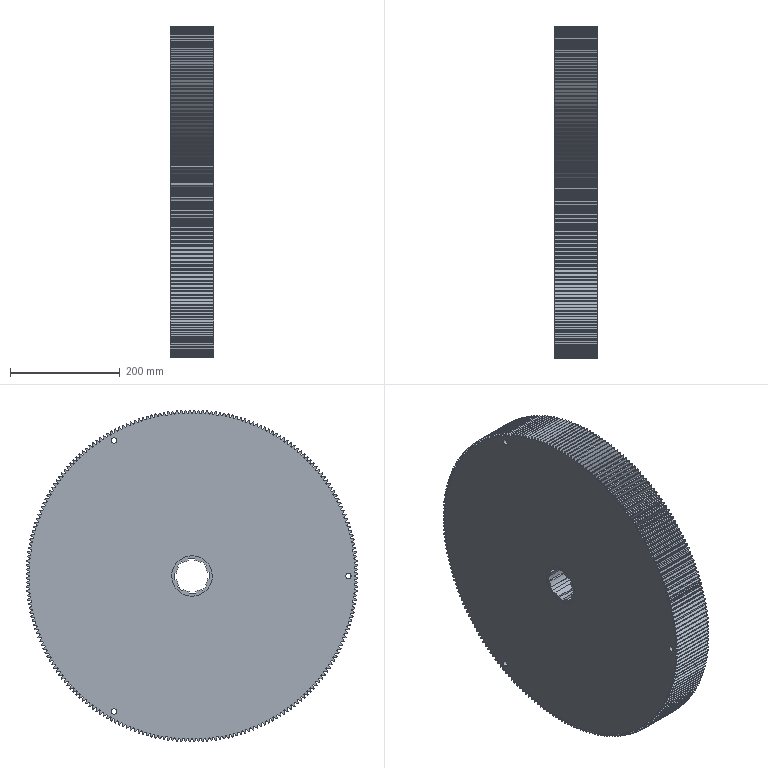Part | SolidWorks | features Punch 2, BaseBody 1, CirPattern 1, HoleWzd 1, ICE 1 | 1 solid | 1018 faces | box 80 x 604.968 x 604.968 mm | volume 22281815 mm3 | cylinder 996 | plane 22 | commonest cylinder face diameters 240 x484 593.748 x241 605 x240 64 x9 58 x8 10 x6